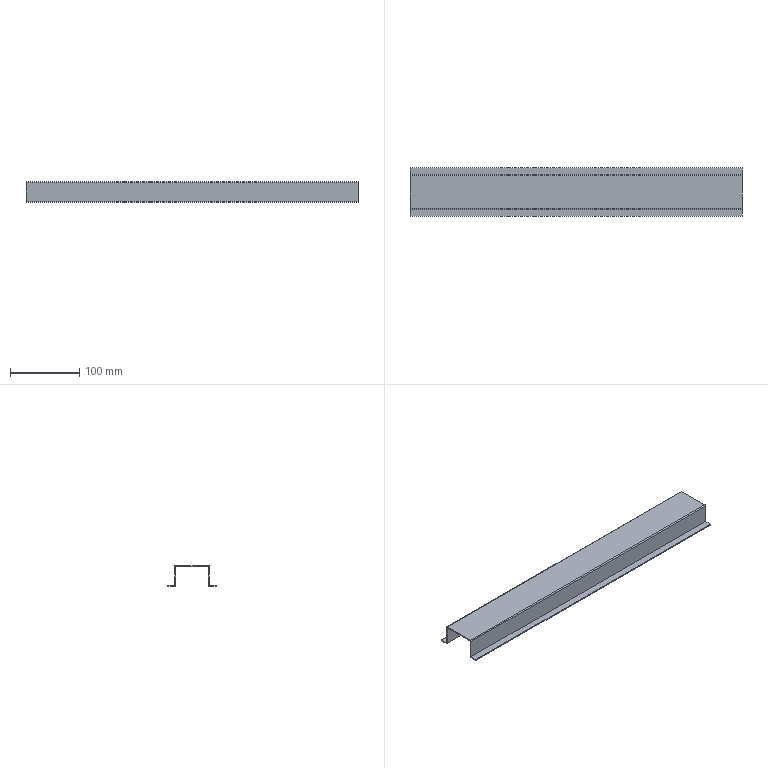Part | STEP file | 1 solid | 18 faces | box 479 x 70 x 30 mm | volume 90339 mm3 | plane 14 | cylinder 4 | commonest cylinder face diameters 3.004 x4
STEP:
#1=CARTESIAN_POINT('',(0.,0.,0.));
#2=DIRECTION('',(0.,0.,1.));
#3=DIRECTION('',(1.,0.,0.));
#4=AXIS2_PLACEMENT_3D('',#1,#2,#3);
#5=CARTESIAN_POINT('',(-1052.573,4254.073,1741.146));
#6=VERTEX_POINT('',#5);
#7=CARTESIAN_POINT('',(-1052.573,4254.073,1768.143));
#8=VERTEX_POINT('',#7);
#9=CARTESIAN_POINT('',(-1052.573,4254.073,1741.146));
#10=DIRECTION('',(0.,0.00002469,1.));
#11=VECTOR('',#10,1.);
#12=LINE('',#9,#11);
#13=CARTESIAN_POINT('',(-1052.573,4302.573,1768.144));
#14=DIRECTION('',(-1.,0.,0.));
#15=DIRECTION('',(0.,0.,1.));
#16=AXIS2_PLACEMENT_3D('',#13,#14,#15);
#17=PLANE('',#16);
#18=CARTESIAN_POINT('',(-26.998,-48.5));
#19=DIRECTION('',(1.,0.00002469));
#20=VECTOR('',#19,1.);
#21=LINE('',#18,#20);
#22=(GEOMETRIC_REPRESENTATION_CONTEXT(2)PARAMETRIC_REPRESENTATION_CONTEXT()REPRESENTATION_CONTEXT('',''));
#23=DEFINITIONAL_REPRESENTATION('',(#21),#22);
#24=PCURVE('',#17,#23);
#25=CARTESIAN_POINT('',(0.,4254.073,0.));
#26=DIRECTION('',(0.,-1.,0.));
#27=DIRECTION('',(0.,0.,-1.));
#28=AXIS2_PLACEMENT_3D('',#25,#26,#27);
#29=PLANE('',#28);
#30=CARTESIAN_POINT('',(-1741.146,-1052.573));
#31=DIRECTION('',(-1.,0.));
#32=VECTOR('',#31,1.);
#33=LINE('',#30,#32);
#34=(GEOMETRIC_REPRESENTATION_CONTEXT(2)PARAMETRIC_REPRESENTATION_CONTEXT()REPRESENTATION_CONTEXT('',''));
#35=DEFINITIONAL_REPRESENTATION('',(#33),#34);
#36=PCURVE('',#29,#35);
#37=SURFACE_CURVE('',#12,(#24,#36),.PCURVE_S1.);
#38=EDGE_CURVE('',#6,#8,#37,.T.);
#39=ORIENTED_EDGE('',*,*,#38,.T.);
#40=CARTESIAN_POINT('',(-1052.573,4301.072,1768.143));
#41=VERTEX_POINT('',#40);
#42=CARTESIAN_POINT('',(-1052.573,4254.073,1768.143));
#43=DIRECTION('',(0.,1.,0.));
#44=VECTOR('',#43,1.);
#45=LINE('',#42,#44);
#46=CARTESIAN_POINT('',(-0.0006667,-48.499));
#47=DIRECTION('',(0.,1.));
#48=VECTOR('',#47,1.);
#49=LINE('',#46,#48);
#50=(GEOMETRIC_REPRESENTATION_CONTEXT(2)PARAMETRIC_REPRESENTATION_CONTEXT()REPRESENTATION_CONTEXT('',''));
#51=DEFINITIONAL_REPRESENTATION('',(#49),#50);
#52=PCURVE('',#17,#51);
#53=CARTESIAN_POINT('',(0.,0.,1768.144));
#54=DIRECTION('',(0.,0.,1.));
#55=DIRECTION('',(1.,0.,0.));
#56=AXIS2_PLACEMENT_3D('',#53,#54,#55);
#57=PLANE('',#56);
#58=CARTESIAN_POINT('',(-1052.573,4254.073));
#59=DIRECTION('',(0.,1.));
#60=VECTOR('',#59,1.);
#61=LINE('',#58,#60);
#62=(GEOMETRIC_REPRESENTATION_CONTEXT(2)PARAMETRIC_REPRESENTATION_CONTEXT()REPRESENTATION_CONTEXT('',''));
#63=DEFINITIONAL_REPRESENTATION('',(#61),#62);
#64=PCURVE('',#57,#63);
#65=SURFACE_CURVE('',#45,(#52,#64),.PCURVE_S1.);
#66=EDGE_CURVE('',#8,#41,#65,.T.);
#67=ORIENTED_EDGE('',*,*,#66,.T.);
#68=CARTESIAN_POINT('',(-1052.573,4301.073,1741.146));
#69=VERTEX_POINT('',#68);
#70=CARTESIAN_POINT('',(-1052.573,4301.073,1741.146));
#71=DIRECTION('',(0.,-0.00002469,1.));
#72=VECTOR('',#71,1.);
#73=LINE('',#70,#72);
#74=CARTESIAN_POINT('',(-26.998,-1.5));
#75=DIRECTION('',(1.,-0.00002469));
#76=VECTOR('',#75,1.);
#77=LINE('',#74,#76);
#78=(GEOMETRIC_REPRESENTATION_CONTEXT(2)PARAMETRIC_REPRESENTATION_CONTEXT()REPRESENTATION_CONTEXT('',''));
#79=DEFINITIONAL_REPRESENTATION('',(#77),#78);
#80=PCURVE('',#17,#79);
#81=CARTESIAN_POINT('',(0.,4301.073,0.));
#82=DIRECTION('',(0.,-1.,0.));
#83=DIRECTION('',(0.,0.,-1.));
#84=AXIS2_PLACEMENT_3D('',#81,#82,#83);
#85=PLANE('',#84);
#86=CARTESIAN_POINT('',(-1741.146,-1052.573));
#87=DIRECTION('',(-1.,0.));
#88=VECTOR('',#87,1.);
#89=LINE('',#86,#88);
#90=(GEOMETRIC_REPRESENTATION_CONTEXT(2)PARAMETRIC_REPRESENTATION_CONTEXT()REPRESENTATION_CONTEXT('',''));
#91=DEFINITIONAL_REPRESENTATION('',(#89),#90);
#92=PCURVE('',#85,#91);
#93=SURFACE_CURVE('',#73,(#80,#92),.PCURVE_S1.);
#94=EDGE_CURVE('',#69,#41,#93,.T.);
#95=ORIENTED_EDGE('',*,*,#94,.F.);
#96=CARTESIAN_POINT('',(-1052.573,4302.575,1739.644));
#97=VERTEX_POINT('',#96);
#98=CARTESIAN_POINT('',(-1052.573,4302.575,1741.146));
#99=DIRECTION('',(-1.,0.,0.));
#100=DIRECTION('',(0.,0.,-1.));
#101=AXIS2_PLACEMENT_3D('',#98,#99,#100);
#102=CIRCLE('',#101,1.502);
#103=CARTESIAN_POINT('',(-26.998,0.002));
#104=DIRECTION('',(-1.,0.));
#105=AXIS2_PLACEMENT_2D('',#103,#104);
#106=CIRCLE('',#105,1.502);
#107=(GEOMETRIC_REPRESENTATION_CONTEXT(2)PARAMETRIC_REPRESENTATION_CONTEXT()REPRESENTATION_CONTEXT('',''));
#108=DEFINITIONAL_REPRESENTATION('',(#106),#107);
#109=PCURVE('',#17,#108);
#110=CARTESIAN_POINT('',(-1052.573,4302.575,1741.146));
#111=DIRECTION('',(1.,0.,0.));
#112=DIRECTION('',(0.,1.,0.));
#113=AXIS2_PLACEMENT_3D('',#110,#111,#112);
#114=CYLINDRICAL_SURFACE('',#113,1.502);
#115=CARTESIAN_POINT('',(4.712,0.));
#116=DIRECTION('',(-1.,0.));
#117=VECTOR('',#116,1.);
#118=LINE('',#115,#117);
#119=(GEOMETRIC_REPRESENTATION_CONTEXT(2)PARAMETRIC_REPRESENTATION_CONTEXT()REPRESENTATION_CONTEXT('',''));
#120=DEFINITIONAL_REPRESENTATION('',(#118),#119);
#121=PCURVE('',#114,#120);
#122=SURFACE_CURVE('',#102,(#109,#121),.PCURVE_S1.);
#123=EDGE_CURVE('',#97,#69,#122,.T.);
#124=ORIENTED_EDGE('',*,*,#123,.F.);
#125=CARTESIAN_POINT('',(-1052.573,4312.573,1739.644));
#126=VERTEX_POINT('',#125);
#127=CARTESIAN_POINT('',(-1052.573,4312.573,1739.644));
#128=DIRECTION('',(0.,-1.,0.));
#129=VECTOR('',#128,1.);
#130=LINE('',#127,#129);
#131=CARTESIAN_POINT('',(-28.5,10.));
#132=DIRECTION('',(0.,-1.));
#133=VECTOR('',#132,1.);
#134=LINE('',#131,#133);
#135=(GEOMETRIC_REPRESENTATION_CONTEXT(2)PARAMETRIC_REPRESENTATION_CONTEXT()REPRESENTATION_CONTEXT('',''));
#136=DEFINITIONAL_REPRESENTATION('',(#134),#135);
#137=PCURVE('',#17,#136);
#138=CARTESIAN_POINT('',(0.,0.,1739.644));
#139=DIRECTION('',(0.,0.,-1.));
#140=DIRECTION('',(-1.,0.,0.));
#141=AXIS2_PLACEMENT_3D('',#138,#139,#140);
#142=PLANE('',#141);
#143=CARTESIAN_POINT('',(1052.573,4312.573));
#144=DIRECTION('',(0.,-1.));
#145=VECTOR('',#144,1.);
#146=LINE('',#143,#145);
#147=(GEOMETRIC_REPRESENTATION_CONTEXT(2)PARAMETRIC_REPRESENTATION_CONTEXT()REPRESENTATION_CONTEXT('',''));
#148=DEFINITIONAL_REPRESENTATION('',(#146),#147);
#149=PCURVE('',#142,#148);
#150=SURFACE_CURVE('',#130,(#137,#149),.PCURVE_S1.);
#151=EDGE_CURVE('',#126,#97,#150,.T.);
#152=ORIENTED_EDGE('',*,*,#151,.F.);
#153=CARTESIAN_POINT('',(-1052.573,4312.573,1741.144));
#154=VERTEX_POINT('',#153);
#155=CARTESIAN_POINT('',(-1052.573,4312.573,1741.144));
#156=DIRECTION('',(0.,0.,-1.));
#157=VECTOR('',#156,1.);
#158=LINE('',#155,#157);
#159=CARTESIAN_POINT('',(-27.,10.));
#160=DIRECTION('',(-1.,0.));
#161=VECTOR('',#160,1.);
#162=LINE('',#159,#161);
#163=(GEOMETRIC_REPRESENTATION_CONTEXT(2)PARAMETRIC_REPRESENTATION_CONTEXT()REPRESENTATION_CONTEXT('',''));
#164=DEFINITIONAL_REPRESENTATION('',(#162),#163);
#165=PCURVE('',#17,#164);
#166=CARTESIAN_POINT('',(-1052.573,4312.573,1739.644));
#167=DIRECTION('',(0.,-1.,0.));
#168=DIRECTION('',(0.,0.,-1.));
#169=AXIS2_PLACEMENT_3D('',#166,#167,#168);
#170=PLANE('',#169);
#171=CARTESIAN_POINT('',(-1.5,0.));
#172=DIRECTION('',(1.,0.));
#173=VECTOR('',#172,1.);
#174=LINE('',#171,#173);
#175=(GEOMETRIC_REPRESENTATION_CONTEXT(2)PARAMETRIC_REPRESENTATION_CONTEXT()REPRESENTATION_CONTEXT('',''));
#176=DEFINITIONAL_REPRESENTATION('',(#174),#175);
#177=PCURVE('',#170,#176);
#178=SURFACE_CURVE('',#158,(#165,#177),.PCURVE_S1.);
#179=EDGE_CURVE('',#154,#126,#178,.T.);
#180=ORIENTED_EDGE('',*,*,#179,.F.);
#181=CARTESIAN_POINT('',(-1052.573,4302.573,1741.144));
#182=VERTEX_POINT('',#181);
#183=CARTESIAN_POINT('',(-1052.573,4312.573,1741.144));
#184=DIRECTION('',(0.,-1.,0.00006667));
#185=VECTOR('',#184,1.);
#186=LINE('',#183,#185);
#187=CARTESIAN_POINT('',(-27.,10.));
#188=DIRECTION('',(0.00006667,-1.));
#189=VECTOR('',#188,1.);
#190=LINE('',#187,#189);
#191=(GEOMETRIC_REPRESENTATION_CONTEXT(2)PARAMETRIC_REPRESENTATION_CONTEXT()REPRESENTATION_CONTEXT('',''));
#192=DEFINITIONAL_REPRESENTATION('',(#190),#191);
#193=PCURVE('',#17,#192);
#194=CARTESIAN_POINT('',(0.,0.,1741.144));
#195=DIRECTION('',(0.,0.,-1.));
#196=DIRECTION('',(-1.,0.,0.));
#197=AXIS2_PLACEMENT_3D('',#194,#195,#196);
#198=PLANE('',#197);
#199=CARTESIAN_POINT('',(1052.573,4312.573));
#200=DIRECTION('',(0.,-1.));
#201=VECTOR('',#200,1.);
#202=LINE('',#199,#201);
#203=(GEOMETRIC_REPRESENTATION_CONTEXT(2)PARAMETRIC_REPRESENTATION_CONTEXT()REPRESENTATION_CONTEXT('',''));
#204=DEFINITIONAL_REPRESENTATION('',(#202),#203);
#205=PCURVE('',#198,#204);
#206=SURFACE_CURVE('',#186,(#193,#205),.PCURVE_S1.);
#207=EDGE_CURVE('',#154,#182,#206,.T.);
#208=ORIENTED_EDGE('',*,*,#207,.T.);
#209=CARTESIAN_POINT('',(-1052.573,4302.573,1768.142));
#210=VERTEX_POINT('',#209);
#211=CARTESIAN_POINT('',(-1052.573,4302.573,1741.144));
#212=DIRECTION('',(0.,-0.00002469,1.));
#213=VECTOR('',#212,1.);
#214=LINE('',#211,#213);
#215=CARTESIAN_POINT('',(-26.999,0.0006667));
#216=DIRECTION('',(1.,-0.00002469));
#217=VECTOR('',#216,1.);
#218=LINE('',#215,#217);
#219=(GEOMETRIC_REPRESENTATION_CONTEXT(2)PARAMETRIC_REPRESENTATION_CONTEXT()REPRESENTATION_CONTEXT('',''));
#220=DEFINITIONAL_REPRESENTATION('',(#218),#219);
#221=PCURVE('',#17,#220);
#222=CARTESIAN_POINT('',(0.,4302.573,0.));
#223=DIRECTION('',(0.,-1.,0.));
#224=DIRECTION('',(0.,0.,-1.));
#225=AXIS2_PLACEMENT_3D('',#222,#223,#224);
#226=PLANE('',#225);
#227=CARTESIAN_POINT('',(-1741.144,-1052.573));
#228=DIRECTION('',(-1.,0.));
#229=VECTOR('',#228,1.);
#230=LINE('',#227,#229);
#231=(GEOMETRIC_REPRESENTATION_CONTEXT(2)PARAMETRIC_REPRESENTATION_CONTEXT()REPRESENTATION_CONTEXT('',''));
#232=DEFINITIONAL_REPRESENTATION('',(#230),#231);
#233=PCURVE('',#226,#232);
#234=SURFACE_CURVE('',#214,(#221,#233),.PCURVE_S1.);
#235=EDGE_CURVE('',#182,#210,#234,.T.);
#236=ORIENTED_EDGE('',*,*,#235,.T.);
#237=CARTESIAN_POINT('',(-1052.573,4301.071,1769.644));
#238=VERTEX_POINT('',#237);
#239=CARTESIAN_POINT('',(-1052.573,4301.071,1768.142));
#240=DIRECTION('',(-1.,0.,0.));
#241=DIRECTION('',(0.,0.,1.));
#242=AXIS2_PLACEMENT_3D('',#239,#240,#241);
#243=CIRCLE('',#242,1.502);
#244=CARTESIAN_POINT('',(-0.002,-1.502));
#245=DIRECTION('',(1.,0.));
#246=AXIS2_PLACEMENT_2D('',#244,#245);
#247=CIRCLE('',#246,1.502);
#248=(GEOMETRIC_REPRESENTATION_CONTEXT(2)PARAMETRIC_REPRESENTATION_CONTEXT()REPRESENTATION_CONTEXT('',''));
#249=DEFINITIONAL_REPRESENTATION('',(#247),#248);
#250=PCURVE('',#17,#249);
#251=CARTESIAN_POINT('',(-573.573,4301.071,1768.142));
#252=DIRECTION('',(-1.,0.,0.));
#253=DIRECTION('',(0.,0.,-1.));
#254=AXIS2_PLACEMENT_3D('',#251,#252,#253);
#255=CYLINDRICAL_SURFACE('',#254,1.502);
#256=CARTESIAN_POINT('',(3.142,479.));
#257=DIRECTION('',(1.,0.));
#258=VECTOR('',#257,1.);
#259=LINE('',#256,#258);
#260=(GEOMETRIC_REPRESENTATION_CONTEXT(2)PARAMETRIC_REPRESENTATION_CONTEXT()REPRESENTATION_CONTEXT('',''));
#261=DEFINITIONAL_REPRESENTATION('',(#259),#260);
#262=PCURVE('',#255,#261);
#263=SURFACE_CURVE('',#243,(#250,#262),.PCURVE_S1.);
#264=EDGE_CURVE('',#238,#210,#263,.T.);
#265=ORIENTED_EDGE('',*,*,#264,.F.);
#266=CARTESIAN_POINT('',(-1052.573,4254.075,1769.644));
#267=VERTEX_POINT('',#266);
#268=CARTESIAN_POINT('',(-1052.573,4254.075,1769.644));
#269=DIRECTION('',(0.,1.,0.));
#270=VECTOR('',#269,1.);
#271=LINE('',#268,#270);
#272=CARTESIAN_POINT('',(1.5,-48.498));
#273=DIRECTION('',(0.,1.));
#274=VECTOR('',#273,1.);
#275=LINE('',#272,#274);
#276=(GEOMETRIC_REPRESENTATION_CONTEXT(2)PARAMETRIC_REPRESENTATION_CONTEXT()REPRESENTATION_CONTEXT('',''));
#277=DEFINITIONAL_REPRESENTATION('',(#275),#276);
#278=PCURVE('',#17,#277);
#279=CARTESIAN_POINT('',(0.,0.,1769.644));
#280=DIRECTION('',(0.,0.,1.));
#281=DIRECTION('',(1.,0.,0.));
#282=AXIS2_PLACEMENT_3D('',#279,#280,#281);
#283=PLANE('',#282);
#284=CARTESIAN_POINT('',(-1052.573,4254.075));
#285=DIRECTION('',(0.,1.));
#286=VECTOR('',#285,1.);
#287=LINE('',#284,#286);
#288=(GEOMETRIC_REPRESENTATION_CONTEXT(2)PARAMETRIC_REPRESENTATION_CONTEXT()REPRESENTATION_CONTEXT('',''));
#289=DEFINITIONAL_REPRESENTATION('',(#287),#288);
#290=PCURVE('',#283,#289);
#291=SURFACE_CURVE('',#271,(#278,#290),.PCURVE_S1.);
#292=EDGE_CURVE('',#267,#238,#291,.T.);
#293=ORIENTED_EDGE('',*,*,#292,.F.);
#294=CARTESIAN_POINT('',(-1052.573,4252.573,1768.142));
#295=VERTEX_POINT('',#294);
#296=CARTESIAN_POINT('',(-1052.573,4254.075,1768.142));
#297=DIRECTION('',(-1.,0.,0.));
#298=DIRECTION('',(0.,-1.,0.));
#299=AXIS2_PLACEMENT_3D('',#296,#297,#298);
#300=CIRCLE('',#299,1.502);
#301=CARTESIAN_POINT('',(-0.002,-48.498));
#302=DIRECTION('',(0.,-1.));
#303=AXIS2_PLACEMENT_2D('',#301,#302);
#304=CIRCLE('',#303,1.502);
#305=(GEOMETRIC_REPRESENTATION_CONTEXT(2)PARAMETRIC_REPRESENTATION_CONTEXT()REPRESENTATION_CONTEXT('',''));
#306=DEFINITIONAL_REPRESENTATION('',(#304),#305);
#307=PCURVE('',#17,#306);
#308=CARTESIAN_POINT('',(-1052.573,4254.075,1768.142));
#309=DIRECTION('',(1.,0.,0.));
#310=DIRECTION('',(0.,0.,-1.));
#311=AXIS2_PLACEMENT_3D('',#308,#309,#310);
#312=CYLINDRICAL_SURFACE('',#311,1.502);
#313=CARTESIAN_POINT('',(4.712,0.));
#314=DIRECTION('',(-1.,0.));
#315=VECTOR('',#314,1.);
#316=LINE('',#313,#315);
#317=(GEOMETRIC_REPRESENTATION_CONTEXT(2)PARAMETRIC_REPRESENTATION_CONTEXT()REPRESENTATION_CONTEXT('',''));
#318=DEFINITIONAL_REPRESENTATION('',(#316),#317);
#319=PCURVE('',#312,#318);
#320=SURFACE_CURVE('',#300,(#307,#319),.PCURVE_S1.);
#321=EDGE_CURVE('',#295,#267,#320,.T.);
#322=ORIENTED_EDGE('',*,*,#321,.F.);
#323=CARTESIAN_POINT('',(-1052.573,4252.572,1741.144));
#324=VERTEX_POINT('',#323);
#325=CARTESIAN_POINT('',(-1052.573,4252.572,1741.144));
#326=DIRECTION('',(0.,0.00002469,1.));
#327=VECTOR('',#326,1.);
#328=LINE('',#325,#327);
#329=CARTESIAN_POINT('',(-26.999,-50.001));
#330=DIRECTION('',(1.,0.00002469));
#331=VECTOR('',#330,1.);
#332=LINE('',#329,#331);
#333=(GEOMETRIC_REPRESENTATION_CONTEXT(2)PARAMETRIC_REPRESENTATION_CONTEXT()REPRESENTATION_CONTEXT('',''));
#334=DEFINITIONAL_REPRESENTATION('',(#332),#333);
#335=PCURVE('',#17,#334);
#336=CARTESIAN_POINT('',(0.,4252.573,0.));
#337=DIRECTION('',(0.,-1.,0.));
#338=DIRECTION('',(0.,0.,-1.));
#339=AXIS2_PLACEMENT_3D('',#336,#337,#338);
#340=PLANE('',#339);
#341=CARTESIAN_POINT('',(-1741.144,-1052.573));
#342=DIRECTION('',(-1.,0.));
#343=VECTOR('',#342,1.);
#344=LINE('',#341,#343);
#345=(GEOMETRIC_REPRESENTATION_CONTEXT(2)PARAMETRIC_REPRESENTATION_CONTEXT()REPRESENTATION_CONTEXT('',''));
#346=DEFINITIONAL_REPRESENTATION('',(#344),#345);
#347=PCURVE('',#340,#346);
#348=SURFACE_CURVE('',#328,(#335,#347),.PCURVE_S1.);
#349=EDGE_CURVE('',#324,#295,#348,.T.);
#350=ORIENTED_EDGE('',*,*,#349,.F.);
#351=CARTESIAN_POINT('',(-1052.573,4242.573,1741.144));
#352=VERTEX_POINT('',#351);
#353=CARTESIAN_POINT('',(-1052.573,4242.573,1741.144));
#354=DIRECTION('',(0.,1.,0.00006667));
#355=VECTOR('',#354,1.);
#356=LINE('',#353,#355);
#357=CARTESIAN_POINT('',(-27.,-60.));
#358=DIRECTION('',(0.00006667,1.));
#359=VECTOR('',#358,1.);
#360=LINE('',#357,#359);
#361=(GEOMETRIC_REPRESENTATION_CONTEXT(2)PARAMETRIC_REPRESENTATION_CONTEXT()REPRESENTATION_CONTEXT('',''));
#362=DEFINITIONAL_REPRESENTATION('',(#360),#361);
#363=PCURVE('',#17,#362);
#364=CARTESIAN_POINT('',(0.,0.,1741.144));
#365=DIRECTION('',(0.,0.,1.));
#366=DIRECTION('',(1.,0.,0.));
#367=AXIS2_PLACEMENT_3D('',#364,#365,#366);
#368=PLANE('',#367);
#369=CARTESIAN_POINT('',(-1052.573,4242.573));
#370=DIRECTION('',(0.,1.));
#371=VECTOR('',#370,1.);
#372=LINE('',#369,#371);
#373=(GEOMETRIC_REPRESENTATION_CONTEXT(2)PARAMETRIC_REPRESENTATION_CONTEXT()REPRESENTATION_CONTEXT('',''));
#374=DEFINITIONAL_REPRESENTATION('',(#372),#373);
#375=PCURVE('',#368,#374);
#376=SURFACE_CURVE('',#356,(#363,#375),.PCURVE_S1.);
#377=EDGE_CURVE('',#352,#324,#376,.T.);
#378=ORIENTED_EDGE('',*,*,#377,.F.);
#379=CARTESIAN_POINT('',(-1052.573,4242.573,1739.644));
#380=VERTEX_POINT('',#379);
#381=CARTESIAN_POINT('',(-1052.573,4242.573,1741.144));
#382=DIRECTION('',(0.,0.,-1.));
#383=VECTOR('',#382,1.);
#384=LINE('',#381,#383);
#385=CARTESIAN_POINT('',(-27.,-60.));
#386=DIRECTION('',(-1.,0.));
#387=VECTOR('',#386,1.);
#388=LINE('',#385,#387);
#389=(GEOMETRIC_REPRESENTATION_CONTEXT(2)PARAMETRIC_REPRESENTATION_CONTEXT()REPRESENTATION_CONTEXT('',''));
#390=DEFINITIONAL_REPRESENTATION('',(#388),#389);
#391=PCURVE('',#17,#390);
#392=CARTESIAN_POINT('',(-1052.573,4242.573,1739.644));
#393=DIRECTION('',(0.,-1.,0.));
#394=DIRECTION('',(0.,0.,-1.));
#395=AXIS2_PLACEMENT_3D('',#392,#393,#394);
#396=PLANE('',#395);
#397=CARTESIAN_POINT('',(-1.5,0.));
#398=DIRECTION('',(1.,0.));
#399=VECTOR('',#398,1.);
#400=LINE('',#397,#399);
#401=(GEOMETRIC_REPRESENTATION_CONTEXT(2)PARAMETRIC_REPRESENTATION_CONTEXT()REPRESENTATION_CONTEXT('',''));
#402=DEFINITIONAL_REPRESENTATION('',(#400),#401);
#403=PCURVE('',#396,#402);
#404=SURFACE_CURVE('',#384,(#391,#403),.PCURVE_S1.);
#405=EDGE_CURVE('',#352,#380,#404,.T.);
#406=ORIENTED_EDGE('',*,*,#405,.T.);
#407=CARTESIAN_POINT('',(-1052.573,4252.571,1739.644));
#408=VERTEX_POINT('',#407);
#409=CARTESIAN_POINT('',(-1052.573,4242.573,1739.644));
#410=DIRECTION('',(0.,1.,0.));
#411=VECTOR('',#410,1.);
#412=LINE('',#409,#411);
#413=CARTESIAN_POINT('',(-28.5,-60.));
#414=DIRECTION('',(0.,1.));
#415=VECTOR('',#414,1.);
#416=LINE('',#413,#415);
#417=(GEOMETRIC_REPRESENTATION_CONTEXT(2)PARAMETRIC_REPRESENTATION_CONTEXT()REPRESENTATION_CONTEXT('',''));
#418=DEFINITIONAL_REPRESENTATION('',(#416),#417);
#419=PCURVE('',#17,#418);
#420=CARTESIAN_POINT('',(0.,0.,1739.644));
#421=DIRECTION('',(0.,0.,1.));
#422=DIRECTION('',(1.,0.,0.));
#423=AXIS2_PLACEMENT_3D('',#420,#421,#422);
#424=PLANE('',#423);
#425=CARTESIAN_POINT('',(-1052.573,4242.573));
#426=DIRECTION('',(0.,1.));
#427=VECTOR('',#426,1.);
#428=LINE('',#425,#427);
#429=(GEOMETRIC_REPRESENTATION_CONTEXT(2)PARAMETRIC_REPRESENTATION_CONTEXT()REPRESENTATION_CONTEXT('',''));
#430=DEFINITIONAL_REPRESENTATION('',(#428),#429);
#431=PCURVE('',#424,#430);
#432=SURFACE_CURVE('',#412,(#419,#431),.PCURVE_S1.);
#433=EDGE_CURVE('',#380,#408,#432,.T.);
#434=ORIENTED_EDGE('',*,*,#433,.T.);
#435=CARTESIAN_POINT('',(-1052.573,4252.571,1741.146));
#436=DIRECTION('',(-1.,0.,0.));
#437=DIRECTION('',(0.,1.,0.));
#438=AXIS2_PLACEMENT_3D('',#435,#436,#437);
#439=CIRCLE('',#438,1.502);
#440=CARTESIAN_POINT('',(-26.998,-50.002));
#441=DIRECTION('',(0.,1.));
#442=AXIS2_PLACEMENT_2D('',#440,#441);
#443=CIRCLE('',#442,1.502);
#444=(GEOMETRIC_REPRESENTATION_CONTEXT(2)PARAMETRIC_REPRESENTATION_CONTEXT()REPRESENTATION_CONTEXT('',''));
#445=DEFINITIONAL_REPRESENTATION('',(#443),#444);
#446=PCURVE('',#17,#445);
#447=CARTESIAN_POINT('',(-573.573,4252.571,1741.146));
#448=DIRECTION('',(-1.,0.,0.));
#449=DIRECTION('',(0.,-1.,0.));
#450=AXIS2_PLACEMENT_3D('',#447,#448,#449);
#451=CYLINDRICAL_SURFACE('',#450,1.502);
#452=CARTESIAN_POINT('',(3.142,479.));
#453=DIRECTION('',(1.,0.));
#454=VECTOR('',#453,1.);
#455=LINE('',#452,#454);
#456=(GEOMETRIC_REPRESENTATION_CONTEXT(2)PARAMETRIC_REPRESENTATION_CONTEXT()REPRESENTATION_CONTEXT('',''));
#457=DEFINITIONAL_REPRESENTATION('',(#455),#456);
#458=PCURVE('',#451,#457);
#459=SURFACE_CURVE('',#439,(#446,#458),.PCURVE_S1.);
#460=EDGE_CURVE('',#6,#408,#459,.T.);
#461=ORIENTED_EDGE('',*,*,#460,.F.);
#462=EDGE_LOOP('',(#39,#67,#95,#124,#152,#180,#208,#236,#265,#293,#322,#350,#378,#406,#434,#461));
#463=FACE_BOUND('',#462,.F.);
#464=ADVANCED_FACE('',(#463),#17,.T.);
#465=CARTESIAN_POINT('',(-573.573,4254.073,1768.143));
#466=VERTEX_POINT('',#465);
#467=CARTESIAN_POINT('',(-573.573,4254.073,1741.146));
#468=VERTEX_POINT('',#467);
#469=CARTESIAN_POINT('',(-573.573,4254.073,1768.143));
#470=DIRECTION('',(0.,-0.00002469,-1.));
#471=VECTOR('',#470,1.);
#472=LINE('',#469,#471);
#473=CARTESIAN_POINT('',(-1768.143,-573.573));
#474=DIRECTION('',(1.,0.));
#475=VECTOR('',#474,1.);
#476=LINE('',#473,#475);
#477=(GEOMETRIC_REPRESENTATION_CONTEXT(2)PARAMETRIC_REPRESENTATION_CONTEXT()REPRESENTATION_CONTEXT('',''));
#478=DEFINITIONAL_REPRESENTATION('',(#476),#477);
#479=PCURVE('',#29,#478);
#480=CARTESIAN_POINT('',(-573.573,4252.573,1768.144));
#481=DIRECTION('',(1.,0.,0.));
#482=DIRECTION('',(0.,0.,-1.));
#483=AXIS2_PLACEMENT_3D('',#480,#481,#482);
#484=PLANE('',#483);
#485=CARTESIAN_POINT('',(0.0006667,1.501));
#486=DIRECTION('',(1.,-0.00002469));
#487=VECTOR('',#486,1.);
#488=LINE('',#485,#487);
#489=(GEOMETRIC_REPRESENTATION_CONTEXT(2)PARAMETRIC_REPRESENTATION_CONTEXT()REPRESENTATION_CONTEXT('',''));
#490=DEFINITIONAL_REPRESENTATION('',(#488),#489);
#491=PCURVE('',#484,#490);
#492=SURFACE_CURVE('',#472,(#479,#491),.PCURVE_S1.);
#493=EDGE_CURVE('',#466,#468,#492,.T.);
#494=ORIENTED_EDGE('',*,*,#493,.F.);
#495=CARTESIAN_POINT('',(-573.573,4254.073,1768.143));
#496=DIRECTION('',(-1.,0.,0.));
#497=VECTOR('',#496,1.);
#498=LINE('',#495,#497);
#499=CARTESIAN_POINT('',(-1768.143,-573.573));
#500=DIRECTION('',(0.,-1.));
#501=VECTOR('',#500,1.);
#502=LINE('',#499,#501);
#503=(GEOMETRIC_REPRESENTATION_CONTEXT(2)PARAMETRIC_REPRESENTATION_CONTEXT()REPRESENTATION_CONTEXT('',''));
#504=DEFINITIONAL_REPRESENTATION('',(#502),#503);
#505=PCURVE('',#29,#504);
#506=CARTESIAN_POINT('',(-573.573,4254.073));
#507=DIRECTION('',(-1.,0.));
#508=VECTOR('',#507,1.);
#509=LINE('',#506,#508);
#510=(GEOMETRIC_REPRESENTATION_CONTEXT(2)PARAMETRIC_REPRESENTATION_CONTEXT()REPRESENTATION_CONTEXT('',''));
#511=DEFINITIONAL_REPRESENTATION('',(#509),#510);
#512=PCURVE('',#57,#511);
#513=SURFACE_CURVE('',#498,(#505,#512),.PCURVE_S1.);
#514=EDGE_CURVE('',#466,#8,#513,.T.);
#515=ORIENTED_EDGE('',*,*,#514,.T.);
#516=ORIENTED_EDGE('',*,*,#38,.F.);
#517=CARTESIAN_POINT('',(-1052.573,4254.073,1741.146));
#518=DIRECTION('',(1.,0.,0.));
#519=VECTOR('',#518,1.);
#520=LINE('',#517,#519);
#521=CARTESIAN_POINT('',(-1741.146,-1052.573));
#522=DIRECTION('',(0.,1.));
#523=VECTOR('',#522,1.);
#524=LINE('',#521,#523);
#525=(GEOMETRIC_REPRESENTATION_CONTEXT(2)PARAMETRIC_REPRESENTATION_CONTEXT()REPRESENTATION_CONTEXT('',''));
#526=DEFINITIONAL_REPRESENTATION('',(#524),#525);
#527=PCURVE('',#29,#526);
#528=CARTESIAN_POINT('',(3.142,479.));
#529=DIRECTION('',(0.,-1.));
#530=VECTOR('',#529,1.);
#531=LINE('',#528,#530);
#532=(GEOMETRIC_REPRESENTATION_CONTEXT(2)PARAMETRIC_REPRESENTATION_CONTEXT()REPRESENTATION_CONTEXT('',''));
#533=DEFINITIONAL_REPRESENTATION('',(#531),#532);
#534=PCURVE('',#451,#533);
#535=SURFACE_CURVE('',#520,(#527,#534),.PCURVE_S1.);
#536=EDGE_CURVE('',#6,#468,#535,.T.);
#537=ORIENTED_EDGE('',*,*,#536,.T.);
#538=EDGE_LOOP('',(#494,#515,#516,#537));
#539=FACE_BOUND('',#538,.F.);
#540=ADVANCED_FACE('',(#539),#29,.F.);
#541=CARTESIAN_POINT('',(-573.573,4252.573,1768.142));
#542=VERTEX_POINT('',#541);
#543=CARTESIAN_POINT('',(-573.573,4252.572,1741.144));
#544=VERTEX_POINT('',#543);
#545=CARTESIAN_POINT('',(-573.573,4252.573,1768.142));
#546=DIRECTION('',(0.,-0.00002469,-1.));
#547=VECTOR('',#546,1.);
#548=LINE('',#545,#547);
#549=CARTESIAN_POINT('',(0.002,0.));
#550=DIRECTION('',(1.,-0.00002469));
#551=VECTOR('',#550,1.);
#552=LINE('',#549,#551);
#553=(GEOMETRIC_REPRESENTATION_CONTEXT(2)PARAMETRIC_REPRESENTATION_CONTEXT()REPRESENTATION_CONTEXT('',''));
#554=DEFINITIONAL_REPRESENTATION('',(#552),#553);
#555=PCURVE('',#484,#554);
#556=CARTESIAN_POINT('',(-1768.142,-573.573));
#557=DIRECTION('',(1.,0.));
#558=VECTOR('',#557,1.);
#559=LINE('',#556,#558);
#560=(GEOMETRIC_REPRESENTATION_CONTEXT(2)PARAMETRIC_REPRESENTATION_CONTEXT()REPRESENTATION_CONTEXT('',''));
#561=DEFINITIONAL_REPRESENTATION('',(#559),#560);
#562=PCURVE('',#340,#561);
#563=SURFACE_CURVE('',#548,(#555,#562),.PCURVE_S1.);
#564=EDGE_CURVE('',#542,#544,#563,.T.);
#565=ORIENTED_EDGE('',*,*,#564,.F.);
#566=CARTESIAN_POINT('',(-573.573,4254.075,1769.644));
#567=VERTEX_POINT('',#566);
#568=CARTESIAN_POINT('',(-573.573,4254.075,1768.142));
#569=DIRECTION('',(1.,0.,0.));
#570=DIRECTION('',(0.,0.,1.));
#571=AXIS2_PLACEMENT_3D('',#568,#569,#570);
#572=CIRCLE('',#571,1.502);
#573=CARTESIAN_POINT('',(0.002,1.502));
#574=DIRECTION('',(-1.,0.));
#575=AXIS2_PLACEMENT_2D('',#573,#574);
#576=CIRCLE('',#575,1.502);
#577=(GEOMETRIC_REPRESENTATION_CONTEXT(2)PARAMETRIC_REPRESENTATION_CONTEXT()REPRESENTATION_CONTEXT('',''));
#578=DEFINITIONAL_REPRESENTATION('',(#576),#577);
#579=PCURVE('',#484,#578);
#580=CARTESIAN_POINT('',(3.142,479.));
#581=DIRECTION('',(1.,0.));
#582=VECTOR('',#581,1.);
#583=LINE('',#580,#582);
#584=(GEOMETRIC_REPRESENTATION_CONTEXT(2)PARAMETRIC_REPRESENTATION_CONTEXT()REPRESENTATION_CONTEXT('',''));
#585=DEFINITIONAL_REPRESENTATION('',(#583),#584);
#586=PCURVE('',#312,#585);
#587=SURFACE_CURVE('',#572,(#579,#586),.PCURVE_S1.);
#588=EDGE_CURVE('',#567,#542,#587,.T.);
#589=ORIENTED_EDGE('',*,*,#588,.F.);
#590=CARTESIAN_POINT('',(-573.573,4301.071,1769.644));
#591=VERTEX_POINT('',#590);
#592=CARTESIAN_POINT('',(-573.573,4301.071,1769.644));
#593=DIRECTION('',(0.,-1.,0.));
#594=VECTOR('',#593,1.);
#595=LINE('',#592,#594);
#596=CARTESIAN_POINT('',(-1.5,48.498));
#597=DIRECTION('',(0.,-1.));
#598=VECTOR('',#597,1.);
#599=LINE('',#596,#598);
#600=(GEOMETRIC_REPRESENTATION_CONTEXT(2)PARAMETRIC_REPRESENTATION_CONTEXT()REPRESENTATION_CONTEXT('',''));
#601=DEFINITIONAL_REPRESENTATION('',(#599),#600);
#602=PCURVE('',#484,#601);
#603=CARTESIAN_POINT('',(-573.573,4301.071));
#604=DIRECTION('',(0.,-1.));
#605=VECTOR('',#604,1.);
#606=LINE('',#603,#605);
#607=(GEOMETRIC_REPRESENTATION_CONTEXT(2)PARAMETRIC_REPRESENTATION_CONTEXT()REPRESENTATION_CONTEXT('',''));
#608=DEFINITIONAL_REPRESENTATION('',(#606),#607);
#609=PCURVE('',#283,#608);
#610=SURFACE_CURVE('',#595,(#602,#609),.PCURVE_S1.);
#611=EDGE_CURVE('',#591,#567,#610,.T.);
#612=ORIENTED_EDGE('',*,*,#611,.F.);
#613=CARTESIAN_POINT('',(-573.573,4302.573,1768.142));
#614=VERTEX_POINT('',#613);
#615=CARTESIAN_POINT('',(-573.573,4301.071,1768.142));
#616=DIRECTION('',(1.,0.,0.));
#617=DIRECTION('',(0.,1.,0.));
#618=AXIS2_PLACEMENT_3D('',#615,#616,#617);
#619=CIRCLE('',#618,1.502);
#620=CARTESIAN_POINT('',(0.002,48.498));
#621=DIRECTION('',(0.,1.));
#622=AXIS2_PLACEMENT_2D('',#620,#621);
#623=CIRCLE('',#622,1.502);
#624=(GEOMETRIC_REPRESENTATION_CONTEXT(2)PARAMETRIC_REPRESENTATION_CONTEXT()REPRESENTATION_CONTEXT('',''));
#625=DEFINITIONAL_REPRESENTATION('',(#623),#624);
#626=PCURVE('',#484,#625);
#627=CARTESIAN_POINT('',(4.712,0.));
#628=DIRECTION('',(-1.,0.));
#629=VECTOR('',#628,1.);
#630=LINE('',#627,#629);
#631=(GEOMETRIC_REPRESENTATION_CONTEXT(2)PARAMETRIC_REPRESENTATION_CONTEXT()REPRESENTATION_CONTEXT('',''));
#632=DEFINITIONAL_REPRESENTATION('',(#630),#631);
#633=PCURVE('',#255,#632);
#634=SURFACE_CURVE('',#619,(#626,#633),.PCURVE_S1.);
#635=EDGE_CURVE('',#614,#591,#634,.T.);
#636=ORIENTED_EDGE('',*,*,#635,.F.);
#637=CARTESIAN_POINT('',(-573.573,4302.573,1741.144));
#638=VERTEX_POINT('',#637);
#639=CARTESIAN_POINT('',(-573.573,4302.573,1768.142));
#640=DIRECTION('',(0.,0.00002469,-1.));
#641=VECTOR('',#640,1.);
#642=LINE('',#639,#641);
#643=CARTESIAN_POINT('',(0.002,50.));
#644=DIRECTION('',(1.,0.00002469));
#645=VECTOR('',#644,1.);
#646=LINE('',#643,#645);
#647=(GEOMETRIC_REPRESENTATION_CONTEXT(2)PARAMETRIC_REPRESENTATION_CONTEXT()REPRESENTATION_CONTEXT('',''));
#648=DEFINITIONAL_REPRESENTATION('',(#646),#647);
#649=PCURVE('',#484,#648);
#650=CARTESIAN_POINT('',(-1768.142,-573.573));
#651=DIRECTION('',(1.,0.));
#652=VECTOR('',#651,1.);
#653=LINE('',#650,#652);
#654=(GEOMETRIC_REPRESENTATION_CONTEXT(2)PARAMETRIC_REPRESENTATION_CONTEXT()REPRESENTATION_CONTEXT('',''));
#655=DEFINITIONAL_REPRESENTATION('',(#653),#654);
#656=PCURVE('',#226,#655);
#657=SURFACE_CURVE('',#642,(#649,#656),.PCURVE_S1.);
#658=EDGE_CURVE('',#614,#638,#657,.T.);
#659=ORIENTED_EDGE('',*,*,#658,.T.);
#660=CARTESIAN_POINT('',(-573.573,4312.573,1741.144));
#661=VERTEX_POINT('',#660);
#662=CARTESIAN_POINT('',(-573.573,4302.573,1741.144));
#663=DIRECTION('',(0.,1.,-0.00006667));
#664=VECTOR('',#663,1.);
#665=LINE('',#662,#664);
#666=CARTESIAN_POINT('',(26.999,50.001));
#667=DIRECTION('',(0.00006667,1.));
#668=VECTOR('',#667,1.);
#669=LINE('',#666,#668);
#670=(GEOMETRIC_REPRESENTATION_CONTEXT(2)PARAMETRIC_REPRESENTATION_CONTEXT()REPRESENTATION_CONTEXT('',''));
#671=DEFINITIONAL_REPRESENTATION('',(#669),#670);
#672=PCURVE('',#484,#671);
#673=CARTESIAN_POINT('',(573.573,4302.573));
#674=DIRECTION('',(0.,1.));
#675=VECTOR('',#674,1.);
#676=LINE('',#673,#675);
#677=(GEOMETRIC_REPRESENTATION_CONTEXT(2)PARAMETRIC_REPRESENTATION_CONTEXT()REPRESENTATION_CONTEXT('',''));
#678=DEFINITIONAL_REPRESENTATION('',(#676),#677);
#679=PCURVE('',#198,#678);
#680=SURFACE_CURVE('',#665,(#672,#679),.PCURVE_S1.);
#681=EDGE_CURVE('',#638,#661,#680,.T.);
#682=ORIENTED_EDGE('',*,*,#681,.T.);
#683=CARTESIAN_POINT('',(-573.573,4312.573,1739.644));
#684=VERTEX_POINT('',#683);
#685=CARTESIAN_POINT('',(-573.573,4312.573,1741.144));
#686=DIRECTION('',(0.,0.,-1.));
#687=VECTOR('',#686,1.);
#688=LINE('',#685,#687);
#689=CARTESIAN_POINT('',(27.,60.));
#690=DIRECTION('',(1.,0.));
#691=VECTOR('',#690,1.);
#692=LINE('',#689,#691);
#693=(GEOMETRIC_REPRESENTATION_CONTEXT(2)PARAMETRIC_REPRESENTATION_CONTEXT()REPRESENTATION_CONTEXT('',''));
#694=DEFINITIONAL_REPRESENTATION('',(#692),#693);
#695=PCURVE('',#484,#694);
#696=CARTESIAN_POINT('',(-1.5,479.));
#697=DIRECTION('',(1.,0.));
#698=VECTOR('',#697,1.);
#699=LINE('',#696,#698);
#700=(GEOMETRIC_REPRESENTATION_CONTEXT(2)PARAMETRIC_REPRESENTATION_CONTEXT()REPRESENTATION_CONTEXT('',''));
#701=DEFINITIONAL_REPRESENTATION('',(#699),#700);
#702=PCURVE('',#170,#701);
#703=SURFACE_CURVE('',#688,(#695,#702),.PCURVE_S1.);
#704=EDGE_CURVE('',#661,#684,#703,.T.);
#705=ORIENTED_EDGE('',*,*,#704,.T.);
#706=CARTESIAN_POINT('',(-573.573,4302.575,1739.644));
#707=VERTEX_POINT('',#706);
#708=CARTESIAN_POINT('',(-573.573,4302.575,1739.644));
#709=DIRECTION('',(0.,1.,0.));
#710=VECTOR('',#709,1.);
#711=LINE('',#708,#710);
#712=CARTESIAN_POINT('',(28.5,50.002));
#713=DIRECTION('',(0.,1.));
#714=VECTOR('',#713,1.);
#715=LINE('',#712,#714);
#716=(GEOMETRIC_REPRESENTATION_CONTEXT(2)PARAMETRIC_REPRESENTATION_CONTEXT()REPRESENTATION_CONTEXT('',''));
#717=DEFINITIONAL_REPRESENTATION('',(#715),#716);
#718=PCURVE('',#484,#717);
#719=CARTESIAN_POINT('',(573.573,4302.575));
#720=DIRECTION('',(0.,1.));
#721=VECTOR('',#720,1.);
#722=LINE('',#719,#721);
#723=(GEOMETRIC_REPRESENTATION_CONTEXT(2)PARAMETRIC_REPRESENTATION_CONTEXT()REPRESENTATION_CONTEXT('',''));
#724=DEFINITIONAL_REPRESENTATION('',(#722),#723);
#725=PCURVE('',#142,#724);
#726=SURFACE_CURVE('',#711,(#718,#725),.PCURVE_S1.);
#727=EDGE_CURVE('',#707,#684,#726,.T.);
#728=ORIENTED_EDGE('',*,*,#727,.F.);
#729=CARTESIAN_POINT('',(-573.573,4301.073,1741.146));
#730=VERTEX_POINT('',#729);
#731=CARTESIAN_POINT('',(-573.573,4302.575,1741.146));
#732=DIRECTION('',(1.,0.,0.));
#733=DIRECTION('',(0.,-1.,0.));
#734=AXIS2_PLACEMENT_3D('',#731,#732,#733);
#735=CIRCLE('',#734,1.502);
#736=CARTESIAN_POINT('',(26.998,50.002));
#737=DIRECTION('',(0.,-1.));
#738=AXIS2_PLACEMENT_2D('',#736,#737);
#739=CIRCLE('',#738,1.502);
#740=(GEOMETRIC_REPRESENTATION_CONTEXT(2)PARAMETRIC_REPRESENTATION_CONTEXT()REPRESENTATION_CONTEXT('',''));
#741=DEFINITIONAL_REPRESENTATION('',(#739),#740);
#742=PCURVE('',#484,#741);
#743=CARTESIAN_POINT('',(3.142,479.));
#744=DIRECTION('',(1.,0.));
#745=VECTOR('',#744,1.);
#746=LINE('',#743,#745);
#747=(GEOMETRIC_REPRESENTATION_CONTEXT(2)PARAMETRIC_REPRESENTATION_CONTEXT()REPRESENTATION_CONTEXT('',''));
#748=DEFINITIONAL_REPRESENTATION('',(#746),#747);
#749=PCURVE('',#114,#748);
#750=SURFACE_CURVE('',#735,(#742,#749),.PCURVE_S1.);
#751=EDGE_CURVE('',#730,#707,#750,.T.);
#752=ORIENTED_EDGE('',*,*,#751,.F.);
#753=CARTESIAN_POINT('',(-573.573,4301.072,1768.143));
#754=VERTEX_POINT('',#753);
#755=CARTESIAN_POINT('',(-573.573,4301.072,1768.143));
#756=DIRECTION('',(0.,0.00002469,-1.));
#757=VECTOR('',#756,1.);
#758=LINE('',#755,#757);
#759=CARTESIAN_POINT('',(0.0006667,48.499));
#760=DIRECTION('',(1.,0.00002469));
#761=VECTOR('',#760,1.);
#762=LINE('',#759,#761);
#763=(GEOMETRIC_REPRESENTATION_CONTEXT(2)PARAMETRIC_REPRESENTATION_CONTEXT()REPRESENTATION_CONTEXT('',''));
#764=DEFINITIONAL_REPRESENTATION('',(#762),#763);
#765=PCURVE('',#484,#764);
#766=CARTESIAN_POINT('',(-1768.143,-573.573));
#767=DIRECTION('',(1.,0.));
#768=VECTOR('',#767,1.);
#769=LINE('',#766,#768);
#770=(GEOMETRIC_REPRESENTATION_CONTEXT(2)PARAMETRIC_REPRESENTATION_CONTEXT()REPRESENTATION_CONTEXT('',''));
#771=DEFINITIONAL_REPRESENTATION('',(#769),#770);
#772=PCURVE('',#85,#771);
#773=SURFACE_CURVE('',#758,(#765,#772),.PCURVE_S1.);
#774=EDGE_CURVE('',#754,#730,#773,.T.);
#775=ORIENTED_EDGE('',*,*,#774,.F.);
#776=CARTESIAN_POINT('',(-573.573,4301.072,1768.143));
#777=DIRECTION('',(0.,-1.,0.));
#778=VECTOR('',#777,1.);
#779=LINE('',#776,#778);
#780=CARTESIAN_POINT('',(0.0006667,48.499));
#781=DIRECTION('',(0.,-1.));
#782=VECTOR('',#781,1.);
#783=LINE('',#780,#782);
#784=(GEOMETRIC_REPRESENTATION_CONTEXT(2)PARAMETRIC_REPRESENTATION_CONTEXT()REPRESENTATION_CONTEXT('',''));
#785=DEFINITIONAL_REPRESENTATION('',(#783),#784);
#786=PCURVE('',#484,#785);
#787=CARTESIAN_POINT('',(-573.573,4301.072));
#788=DIRECTION('',(0.,-1.));
#789=VECTOR('',#788,1.);
#790=LINE('',#787,#789);
#791=(GEOMETRIC_REPRESENTATION_CONTEXT(2)PARAMETRIC_REPRESENTATION_CONTEXT()REPRESENTATION_CONTEXT('',''));
#792=DEFINITIONAL_REPRESENTATION('',(#790),#791);
#793=PCURVE('',#57,#792);
#794=SURFACE_CURVE('',#779,(#786,#793),.PCURVE_S1.);
#795=EDGE_CURVE('',#754,#466,#794,.T.);
#796=ORIENTED_EDGE('',*,*,#795,.T.);
#797=ORIENTED_EDGE('',*,*,#493,.T.);
#798=CARTESIAN_POINT('',(-573.573,4252.571,1739.644));
#799=VERTEX_POINT('',#798);
#800=CARTESIAN_POINT('',(-573.573,4252.571,1741.146));
#801=DIRECTION('',(1.,0.,0.));
#802=DIRECTION('',(0.,0.,-1.));
#803=AXIS2_PLACEMENT_3D('',#800,#801,#802);
#804=CIRCLE('',#803,1.502);
#805=CARTESIAN_POINT('',(26.998,-0.002));
#806=DIRECTION('',(1.,0.));
#807=AXIS2_PLACEMENT_2D('',#805,#806);
#808=CIRCLE('',#807,1.502);
#809=(GEOMETRIC_REPRESENTATION_CONTEXT(2)PARAMETRIC_REPRESENTATION_CONTEXT()REPRESENTATION_CONTEXT('',''));
#810=DEFINITIONAL_REPRESENTATION('',(#808),#809);
#811=PCURVE('',#484,#810);
#812=CARTESIAN_POINT('',(4.712,0.));
#813=DIRECTION('',(-1.,0.));
#814=VECTOR('',#813,1.);
#815=LINE('',#812,#814);
#816=(GEOMETRIC_REPRESENTATION_CONTEXT(2)PARAMETRIC_REPRESENTATION_CONTEXT()REPRESENTATION_CONTEXT('',''));
#817=DEFINITIONAL_REPRESENTATION('',(#815),#816);
#818=PCURVE('',#451,#817);
#819=SURFACE_CURVE('',#804,(#811,#818),.PCURVE_S1.);
#820=EDGE_CURVE('',#799,#468,#819,.T.);
#821=ORIENTED_EDGE('',*,*,#820,.F.);
#822=CARTESIAN_POINT('',(-573.573,4242.573,1739.644));
#823=VERTEX_POINT('',#822);
#824=CARTESIAN_POINT('',(-573.573,4252.571,1739.644));
#825=DIRECTION('',(0.,-1.,0.));
#826=VECTOR('',#825,1.);
#827=LINE('',#824,#826);
#828=CARTESIAN_POINT('',(28.5,-0.002));
#829=DIRECTION('',(0.,-1.));
#830=VECTOR('',#829,1.);
#831=LINE('',#828,#830);
#832=(GEOMETRIC_REPRESENTATION_CONTEXT(2)PARAMETRIC_REPRESENTATION_CONTEXT()REPRESENTATION_CONTEXT('',''));
#833=DEFINITIONAL_REPRESENTATION('',(#831),#832);
#834=PCURVE('',#484,#833);
#835=CARTESIAN_POINT('',(-573.573,4252.571));
#836=DIRECTION('',(0.,-1.));
#837=VECTOR('',#836,1.);
#838=LINE('',#835,#837);
#839=(GEOMETRIC_REPRESENTATION_CONTEXT(2)PARAMETRIC_REPRESENTATION_CONTEXT()REPRESENTATION_CONTEXT('',''));
#840=DEFINITIONAL_REPRESENTATION('',(#838),#839);
#841=PCURVE('',#424,#840);
#842=SURFACE_CURVE('',#827,(#834,#841),.PCURVE_S1.);
#843=EDGE_CURVE('',#799,#823,#842,.T.);
#844=ORIENTED_EDGE('',*,*,#843,.T.);
#845=CARTESIAN_POINT('',(-573.573,4242.573,1741.144));
#846=VERTEX_POINT('',#845);
#847=CARTESIAN_POINT('',(-573.573,4242.573,1741.144));
#848=DIRECTION('',(0.,0.,-1.));
#849=VECTOR('',#848,1.);
#850=LINE('',#847,#849);
#851=CARTESIAN_POINT('',(27.,-10.));
#852=DIRECTION('',(1.,0.));
#853=VECTOR('',#852,1.);
#854=LINE('',#851,#853);
#855=(GEOMETRIC_REPRESENTATION_CONTEXT(2)PARAMETRIC_REPRESENTATION_CONTEXT()REPRESENTATION_CONTEXT('',''));
#856=DEFINITIONAL_REPRESENTATION('',(#854),#855);
#857=PCURVE('',#484,#856);
#858=CARTESIAN_POINT('',(-1.5,479.));
#859=DIRECTION('',(1.,0.));
#860=VECTOR('',#859,1.);
#861=LINE('',#858,#860);
#862=(GEOMETRIC_REPRESENTATION_CONTEXT(2)PARAMETRIC_REPRESENTATION_CONTEXT()REPRESENTATION_CONTEXT('',''));
#863=DEFINITIONAL_REPRESENTATION('',(#861),#862);
#864=PCURVE('',#396,#863);
#865=SURFACE_CURVE('',#850,(#857,#864),.PCURVE_S1.);
#866=EDGE_CURVE('',#846,#823,#865,.T.);
#867=ORIENTED_EDGE('',*,*,#866,.F.);
#868=CARTESIAN_POINT('',(-573.573,4252.572,1741.144));
#869=DIRECTION('',(0.,-1.,-0.00006667));
#870=VECTOR('',#869,1.);
#871=LINE('',#868,#870);
#872=CARTESIAN_POINT('',(26.999,-0.0006667));
#873=DIRECTION('',(0.00006667,-1.));
#874=VECTOR('',#873,1.);
#875=LINE('',#872,#874);
#876=(GEOMETRIC_REPRESENTATION_CONTEXT(2)PARAMETRIC_REPRESENTATION_CONTEXT()REPRESENTATION_CONTEXT('',''));
#877=DEFINITIONAL_REPRESENTATION('',(#875),#876);
#878=PCURVE('',#484,#877);
#879=CARTESIAN_POINT('',(-573.573,4252.572));
#880=DIRECTION('',(0.,-1.));
#881=VECTOR('',#880,1.);
#882=LINE('',#879,#881);
#883=(GEOMETRIC_REPRESENTATION_CONTEXT(2)PARAMETRIC_REPRESENTATION_CONTEXT()REPRESENTATION_CONTEXT('',''));
#884=DEFINITIONAL_REPRESENTATION('',(#882),#883);
#885=PCURVE('',#368,#884);
#886=SURFACE_CURVE('',#871,(#878,#885),.PCURVE_S1.);
#887=EDGE_CURVE('',#544,#846,#886,.T.);
#888=ORIENTED_EDGE('',*,*,#887,.F.);
#889=EDGE_LOOP('',(#565,#589,#612,#636,#659,#682,#705,#728,#752,#775,#796,#797,#821,#844,#867,#888));
#890=FACE_BOUND('',#889,.F.);
#891=ADVANCED_FACE('',(#890),#484,.T.);
#892=ORIENTED_EDGE('',*,*,#564,.F.);
#893=CARTESIAN_POINT('',(-1052.573,4252.573,1768.142));
#894=DIRECTION('',(1.,0.,0.));
#895=VECTOR('',#894,1.);
#896=LINE('',#893,#895);
#897=CARTESIAN_POINT('',(-1768.142,-1052.573));
#898=DIRECTION('',(0.,1.));
#899=VECTOR('',#898,1.);
#900=LINE('',#897,#899);
#901=(GEOMETRIC_REPRESENTATION_CONTEXT(2)PARAMETRIC_REPRESENTATION_CONTEXT()REPRESENTATION_CONTEXT('',''));
#902=DEFINITIONAL_REPRESENTATION('',(#900),#901);
#903=PCURVE('',#340,#902);
#904=CARTESIAN_POINT('',(4.712,0.));
#905=DIRECTION('',(0.,1.));
#906=VECTOR('',#905,1.);
#907=LINE('',#904,#906);
#908=(GEOMETRIC_REPRESENTATION_CONTEXT(2)PARAMETRIC_REPRESENTATION_CONTEXT()REPRESENTATION_CONTEXT('',''));
#909=DEFINITIONAL_REPRESENTATION('',(#907),#908);
#910=PCURVE('',#312,#909);
#911=SURFACE_CURVE('',#896,(#903,#910),.PCURVE_S1.);
#912=EDGE_CURVE('',#295,#542,#911,.T.);
#913=ORIENTED_EDGE('',*,*,#912,.F.);
#914=ORIENTED_EDGE('',*,*,#349,.F.);
#915=CARTESIAN_POINT('',(-573.573,4252.572,1741.144));
#916=DIRECTION('',(-1.,0.,0.));
#917=VECTOR('',#916,1.);
#918=LINE('',#915,#917);
#919=CARTESIAN_POINT('',(-1741.144,-573.573));
#920=DIRECTION('',(0.,-1.));
#921=VECTOR('',#920,1.);
#922=LINE('',#919,#921);
#923=(GEOMETRIC_REPRESENTATION_CONTEXT(2)PARAMETRIC_REPRESENTATION_CONTEXT()REPRESENTATION_CONTEXT('',''));
#924=DEFINITIONAL_REPRESENTATION('',(#922),#923);
#925=PCURVE('',#340,#924);
#926=CARTESIAN_POINT('',(-573.573,4252.572));
#927=DIRECTION('',(-1.,0.));
#928=VECTOR('',#927,1.);
#929=LINE('',#926,#928);
#930=(GEOMETRIC_REPRESENTATION_CONTEXT(2)PARAMETRIC_REPRESENTATION_CONTEXT()REPRESENTATION_CONTEXT('',''));
#931=DEFINITIONAL_REPRESENTATION('',(#929),#930);
#932=PCURVE('',#368,#931);
#933=SURFACE_CURVE('',#918,(#925,#932),.PCURVE_S1.);
#934=EDGE_CURVE('',#544,#324,#933,.T.);
#935=ORIENTED_EDGE('',*,*,#934,.F.);
#936=EDGE_LOOP('',(#892,#913,#914,#935));
#937=FACE_BOUND('',#936,.T.);
#938=ADVANCED_FACE('',(#937),#340,.T.);
#939=ORIENTED_EDGE('',*,*,#934,.T.);
#940=ORIENTED_EDGE('',*,*,#377,.F.);
#941=CARTESIAN_POINT('',(-573.573,4242.573,1741.144));
#942=DIRECTION('',(-1.,0.,0.));
#943=VECTOR('',#942,1.);
#944=LINE('',#941,#943);
#945=CARTESIAN_POINT('',(-573.573,4242.573));
#946=DIRECTION('',(-1.,0.));
#947=VECTOR('',#946,1.);
#948=LINE('',#945,#947);
#949=(GEOMETRIC_REPRESENTATION_CONTEXT(2)PARAMETRIC_REPRESENTATION_CONTEXT()REPRESENTATION_CONTEXT('',''));
#950=DEFINITIONAL_REPRESENTATION('',(#948),#949);
#951=PCURVE('',#368,#950);
#952=CARTESIAN_POINT('',(-1.5,479.));
#953=DIRECTION('',(0.,-1.));
#954=VECTOR('',#953,1.);
#955=LINE('',#952,#954);
#956=(GEOMETRIC_REPRESENTATION_CONTEXT(2)PARAMETRIC_REPRESENTATION_CONTEXT()REPRESENTATION_CONTEXT('',''));
#957=DEFINITIONAL_REPRESENTATION('',(#955),#956);
#958=PCURVE('',#396,#957);
#959=SURFACE_CURVE('',#944,(#951,#958),.PCURVE_S1.);
#960=EDGE_CURVE('',#846,#352,#959,.T.);
#961=ORIENTED_EDGE('',*,*,#960,.F.);
#962=ORIENTED_EDGE('',*,*,#887,.F.);
#963=EDGE_LOOP('',(#939,#940,#961,#962));
#964=FACE_BOUND('',#963,.T.);
#965=ADVANCED_FACE('',(#964),#368,.T.);
#966=ORIENTED_EDGE('',*,*,#960,.F.);
#967=ORIENTED_EDGE('',*,*,#866,.T.);
#968=CARTESIAN_POINT('',(-573.573,4242.573,1739.644));
#969=DIRECTION('',(-1.,0.,0.));
#970=VECTOR('',#969,1.);
#971=LINE('',#968,#970);
#972=CARTESIAN_POINT('',(0.,479.));
#973=DIRECTION('',(0.,-1.));
#974=VECTOR('',#973,1.);
#975=LINE('',#972,#974);
#976=(GEOMETRIC_REPRESENTATION_CONTEXT(2)PARAMETRIC_REPRESENTATION_CONTEXT()REPRESENTATION_CONTEXT('',''));
#977=DEFINITIONAL_REPRESENTATION('',(#975),#976);
#978=PCURVE('',#396,#977);
#979=CARTESIAN_POINT('',(-573.573,4242.573));
#980=DIRECTION('',(-1.,0.));
#981=VECTOR('',#980,1.);
#982=LINE('',#979,#981);
#983=(GEOMETRIC_REPRESENTATION_CONTEXT(2)PARAMETRIC_REPRESENTATION_CONTEXT()REPRESENTATION_CONTEXT('',''));
#984=DEFINITIONAL_REPRESENTATION('',(#982),#983);
#985=PCURVE('',#424,#984);
#986=SURFACE_CURVE('',#971,(#978,#985),.PCURVE_S1.);
#987=EDGE_CURVE('',#823,#380,#986,.T.);
#988=ORIENTED_EDGE('',*,*,#987,.T.);
#989=ORIENTED_EDGE('',*,*,#405,.F.);
#990=EDGE_LOOP('',(#966,#967,#988,#989));
#991=FACE_BOUND('',#990,.F.);
#992=ADVANCED_FACE('',(#991),#396,.T.);
#993=CARTESIAN_POINT('',(-573.573,4252.571,1739.644));
#994=DIRECTION('',(-1.,0.,0.));
#995=VECTOR('',#994,1.);
#996=LINE('',#993,#995);
#997=CARTESIAN_POINT('',(-573.573,4252.571));
#998=DIRECTION('',(-1.,0.));
#999=VECTOR('',#998,1.);
#1000=LINE('',#997,#999);
#1001=(GEOMETRIC_REPRESENTATION_CONTEXT(2)PARAMETRIC_REPRESENTATION_CONTEXT()REPRESENTATION_CONTEXT('',''));
#1002=DEFINITIONAL_REPRESENTATION('',(#1000),#1001);
#1003=PCURVE('',#424,#1002);
#1004=CARTESIAN_POINT('',(4.712,0.));
#1005=DIRECTION('',(0.,1.));
#1006=VECTOR('',#1005,1.);
#1007=LINE('',#1004,#1006);
#1008=(GEOMETRIC_REPRESENTATION_CONTEXT(2)PARAMETRIC_REPRESENTATION_CONTEXT()REPRESENTATION_CONTEXT('',''));
#1009=DEFINITIONAL_REPRESENTATION('',(#1007),#1008);
#1010=PCURVE('',#451,#1009);
#1011=SURFACE_CURVE('',#996,(#1003,#1010),.PCURVE_S1.);
#1012=EDGE_CURVE('',#799,#408,#1011,.T.);
#1013=ORIENTED_EDGE('',*,*,#1012,.T.);
#1014=ORIENTED_EDGE('',*,*,#433,.F.);
#1015=ORIENTED_EDGE('',*,*,#987,.F.);
#1016=ORIENTED_EDGE('',*,*,#843,.F.);
#1017=EDGE_LOOP('',(#1013,#1014,#1015,#1016));
#1018=FACE_BOUND('',#1017,.F.);
#1019=ADVANCED_FACE('',(#1018),#424,.F.);
#1020=ORIENTED_EDGE('',*,*,#820,.F.);
#1021=ORIENTED_EDGE('',*,*,#1012,.T.);
#1022=ORIENTED_EDGE('',*,*,#460,.F.);
#1023=ORIENTED_EDGE('',*,*,#536,.T.);
#1024=EDGE_LOOP('',(#1020,#1021,#1022,#1023));
#1025=FACE_BOUND('',#1024,.T.);
#1026=ADVANCED_FACE('',(#1025),#451,.T.);
#1027=ORIENTED_EDGE('',*,*,#321,.F.);
#1028=ORIENTED_EDGE('',*,*,#912,.T.);
#1029=ORIENTED_EDGE('',*,*,#588,.F.);
#1030=CARTESIAN_POINT('',(-573.573,4254.075,1769.644));
#1031=DIRECTION('',(-1.,0.,0.));
#1032=VECTOR('',#1031,1.);
#1033=LINE('',#1030,#1032);
#1034=CARTESIAN_POINT('',(3.142,479.));
#1035=DIRECTION('',(0.,-1.));
#1036=VECTOR('',#1035,1.);
#1037=LINE('',#1034,#1036);
#1038=(GEOMETRIC_REPRESENTATION_CONTEXT(2)PARAMETRIC_REPRESENTATION_CONTEXT()REPRESENTATION_CONTEXT('',''));
#1039=DEFINITIONAL_REPRESENTATION('',(#1037),#1038);
#1040=PCURVE('',#312,#1039);
#1041=CARTESIAN_POINT('',(-573.573,4254.075));
#1042=DIRECTION('',(-1.,0.));
#1043=VECTOR('',#1042,1.);
#1044=LINE('',#1041,#1043);
#1045=(GEOMETRIC_REPRESENTATION_CONTEXT(2)PARAMETRIC_REPRESENTATION_CONTEXT()REPRESENTATION_CONTEXT('',''));
#1046=DEFINITIONAL_REPRESENTATION('',(#1044),#1045);
#1047=PCURVE('',#283,#1046);
#1048=SURFACE_CURVE('',#1033,(#1040,#1047),.PCURVE_S1.);
#1049=EDGE_CURVE('',#567,#267,#1048,.T.);
#1050=ORIENTED_EDGE('',*,*,#1049,.T.);
#1051=EDGE_LOOP('',(#1027,#1028,#1029,#1050));
#1052=FACE_BOUND('',#1051,.T.);
#1053=ADVANCED_FACE('',(#1052),#312,.T.);
#1054=ORIENTED_EDGE('',*,*,#611,.T.);
#1055=ORIENTED_EDGE('',*,*,#1049,.T.);
#1056=ORIENTED_EDGE('',*,*,#292,.T.);
#1057=CARTESIAN_POINT('',(-1052.573,4301.071,1769.644));
#1058=DIRECTION('',(1.,0.,0.));
#1059=VECTOR('',#1058,1.);
#1060=LINE('',#1057,#1059);
#1061=CARTESIAN_POINT('',(-1052.573,4301.071));
#1062=DIRECTION('',(1.,0.));
#1063=VECTOR('',#1062,1.);
#1064=LINE('',#1061,#1063);
#1065=(GEOMETRIC_REPRESENTATION_CONTEXT(2)PARAMETRIC_REPRESENTATION_CONTEXT()REPRESENTATION_CONTEXT('',''));
#1066=DEFINITIONAL_REPRESENTATION('',(#1064),#1065);
#1067=PCURVE('',#283,#1066);
#1068=CARTESIAN_POINT('',(3.142,479.));
#1069=DIRECTION('',(0.,-1.));
#1070=VECTOR('',#1069,1.);
#1071=LINE('',#1068,#1070);
#1072=(GEOMETRIC_REPRESENTATION_CONTEXT(2)PARAMETRIC_REPRESENTATION_CONTEXT()REPRESENTATION_CONTEXT('',''));
#1073=DEFINITIONAL_REPRESENTATION('',(#1071),#1072);
#1074=PCURVE('',#255,#1073);
#1075=SURFACE_CURVE('',#1060,(#1067,#1074),.PCURVE_S1.);
#1076=EDGE_CURVE('',#238,#591,#1075,.T.);
#1077=ORIENTED_EDGE('',*,*,#1076,.T.);
#1078=EDGE_LOOP('',(#1054,#1055,#1056,#1077));
#1079=FACE_BOUND('',#1078,.F.);
#1080=ADVANCED_FACE('',(#1079),#283,.T.);
#1081=ORIENTED_EDGE('',*,*,#635,.F.);
#1082=CARTESIAN_POINT('',(-573.573,4302.573,1768.142));
#1083=DIRECTION('',(-1.,0.,0.));
#1084=VECTOR('',#1083,1.);
#1085=LINE('',#1082,#1084);
#1086=CARTESIAN_POINT('',(4.712,0.));
#1087=DIRECTION('',(0.,1.));
#1088=VECTOR('',#1087,1.);
#1089=LINE('',#1086,#1088);
#1090=(GEOMETRIC_REPRESENTATION_CONTEXT(2)PARAMETRIC_REPRESENTATION_CONTEXT()REPRESENTATION_CONTEXT('',''));
#1091=DEFINITIONAL_REPRESENTATION('',(#1089),#1090);
#1092=PCURVE('',#255,#1091);
#1093=CARTESIAN_POINT('',(-1768.142,-573.573));
#1094=DIRECTION('',(0.,-1.));
#1095=VECTOR('',#1094,1.);
#1096=LINE('',#1093,#1095);
#1097=(GEOMETRIC_REPRESENTATION_CONTEXT(2)PARAMETRIC_REPRESENTATION_CONTEXT()REPRESENTATION_CONTEXT('',''));
#1098=DEFINITIONAL_REPRESENTATION('',(#1096),#1097);
#1099=PCURVE('',#226,#1098);
#1100=SURFACE_CURVE('',#1085,(#1092,#1099),.PCURVE_S1.);
#1101=EDGE_CURVE('',#614,#210,#1100,.T.);
#1102=ORIENTED_EDGE('',*,*,#1101,.T.);
#1103=ORIENTED_EDGE('',*,*,#264,.F.);
#1104=ORIENTED_EDGE('',*,*,#1076,.T.);
#1105=EDGE_LOOP('',(#1081,#1102,#1103,#1104));
#1106=FACE_BOUND('',#1105,.T.);
#1107=ADVANCED_FACE('',(#1106),#255,.T.);
#1108=CARTESIAN_POINT('',(-1052.573,4302.573,1741.144));
#1109=DIRECTION('',(1.,0.,0.));
#1110=VECTOR('',#1109,1.);
#1111=LINE('',#1108,#1110);
#1112=CARTESIAN_POINT('',(-1741.144,-1052.573));
#1113=DIRECTION('',(0.,1.));
#1114=VECTOR('',#1113,1.);
#1115=LINE('',#1112,#1114);
#1116=(GEOMETRIC_REPRESENTATION_CONTEXT(2)PARAMETRIC_REPRESENTATION_CONTEXT()REPRESENTATION_CONTEXT('',''));
#1117=DEFINITIONAL_REPRESENTATION('',(#1115),#1116);
#1118=PCURVE('',#226,#1117);
#1119=CARTESIAN_POINT('',(1052.573,4302.573));
#1120=DIRECTION('',(-1.,0.));
#1121=VECTOR('',#1120,1.);
#1122=LINE('',#1119,#1121);
#1123=(GEOMETRIC_REPRESENTATION_CONTEXT(2)PARAMETRIC_REPRESENTATION_CONTEXT()REPRESENTATION_CONTEXT('',''));
#1124=DEFINITIONAL_REPRESENTATION('',(#1122),#1123);
#1125=PCURVE('',#198,#1124);
#1126=SURFACE_CURVE('',#1111,(#1118,#1125),.PCURVE_S1.);
#1127=EDGE_CURVE('',#182,#638,#1126,.T.);
#1128=ORIENTED_EDGE('',*,*,#1127,.T.);
#1129=ORIENTED_EDGE('',*,*,#658,.F.);
#1130=ORIENTED_EDGE('',*,*,#1101,.T.);
#1131=ORIENTED_EDGE('',*,*,#235,.F.);
#1132=EDGE_LOOP('',(#1128,#1129,#1130,#1131));
#1133=FACE_BOUND('',#1132,.F.);
#1134=ADVANCED_FACE('',(#1133),#226,.F.);
#1135=ORIENTED_EDGE('',*,*,#1127,.F.);
#1136=ORIENTED_EDGE('',*,*,#207,.F.);
#1137=CARTESIAN_POINT('',(-573.573,4312.573,1741.144));
#1138=DIRECTION('',(-1.,0.,0.));
#1139=VECTOR('',#1138,1.);
#1140=LINE('',#1137,#1139);
#1141=CARTESIAN_POINT('',(573.573,4312.573));
#1142=DIRECTION('',(1.,0.));
#1143=VECTOR('',#1142,1.);
#1144=LINE('',#1141,#1143);
#1145=(GEOMETRIC_REPRESENTATION_CONTEXT(2)PARAMETRIC_REPRESENTATION_CONTEXT()REPRESENTATION_CONTEXT('',''));
#1146=DEFINITIONAL_REPRESENTATION('',(#1144),#1145);
#1147=PCURVE('',#198,#1146);
#1148=CARTESIAN_POINT('',(-1.5,479.));
#1149=DIRECTION('',(0.,-1.));
#1150=VECTOR('',#1149,1.);
#1151=LINE('',#1148,#1150);
#1152=(GEOMETRIC_REPRESENTATION_CONTEXT(2)PARAMETRIC_REPRESENTATION_CONTEXT()REPRESENTATION_CONTEXT('',''));
#1153=DEFINITIONAL_REPRESENTATION('',(#1151),#1152);
#1154=PCURVE('',#170,#1153);
#1155=SURFACE_CURVE('',#1140,(#1147,#1154),.PCURVE_S1.);
#1156=EDGE_CURVE('',#661,#154,#1155,.T.);
#1157=ORIENTED_EDGE('',*,*,#1156,.F.);
#1158=ORIENTED_EDGE('',*,*,#681,.F.);
#1159=EDGE_LOOP('',(#1135,#1136,#1157,#1158));
#1160=FACE_BOUND('',#1159,.F.);
#1161=ADVANCED_FACE('',(#1160),#198,.F.);
#1162=ORIENTED_EDGE('',*,*,#1156,.T.);
#1163=ORIENTED_EDGE('',*,*,#179,.T.);
#1164=CARTESIAN_POINT('',(-573.573,4312.573,1739.644));
#1165=DIRECTION('',(-1.,0.,0.));
#1166=VECTOR('',#1165,1.);
#1167=LINE('',#1164,#1166);
#1168=CARTESIAN_POINT('',(0.,479.));
#1169=DIRECTION('',(0.,-1.));
#1170=VECTOR('',#1169,1.);
#1171=LINE('',#1168,#1170);
#1172=(GEOMETRIC_REPRESENTATION_CONTEXT(2)PARAMETRIC_REPRESENTATION_CONTEXT()REPRESENTATION_CONTEXT('',''));
#1173=DEFINITIONAL_REPRESENTATION('',(#1171),#1172);
#1174=PCURVE('',#170,#1173);
#1175=CARTESIAN_POINT('',(573.573,4312.573));
#1176=DIRECTION('',(1.,0.));
#1177=VECTOR('',#1176,1.);
#1178=LINE('',#1175,#1177);
#1179=(GEOMETRIC_REPRESENTATION_CONTEXT(2)PARAMETRIC_REPRESENTATION_CONTEXT()REPRESENTATION_CONTEXT('',''));
#1180=DEFINITIONAL_REPRESENTATION('',(#1178),#1179);
#1181=PCURVE('',#142,#1180);
#1182=SURFACE_CURVE('',#1167,(#1174,#1181),.PCURVE_S1.);
#1183=EDGE_CURVE('',#684,#126,#1182,.T.);
#1184=ORIENTED_EDGE('',*,*,#1183,.F.);
#1185=ORIENTED_EDGE('',*,*,#704,.F.);
#1186=EDGE_LOOP('',(#1162,#1163,#1184,#1185));
#1187=FACE_BOUND('',#1186,.F.);
#1188=ADVANCED_FACE('',(#1187),#170,.F.);
#1189=ORIENTED_EDGE('',*,*,#727,.T.);
#1190=ORIENTED_EDGE('',*,*,#1183,.T.);
#1191=ORIENTED_EDGE('',*,*,#151,.T.);
#1192=CARTESIAN_POINT('',(-1052.573,4302.575,1739.644));
#1193=DIRECTION('',(1.,0.,0.));
#1194=VECTOR('',#1193,1.);
#1195=LINE('',#1192,#1194);
#1196=CARTESIAN_POINT('',(1052.573,4302.575));
#1197=DIRECTION('',(-1.,0.));
#1198=VECTOR('',#1197,1.);
#1199=LINE('',#1196,#1198);
#1200=(GEOMETRIC_REPRESENTATION_CONTEXT(2)PARAMETRIC_REPRESENTATION_CONTEXT()REPRESENTATION_CONTEXT('',''));
#1201=DEFINITIONAL_REPRESENTATION('',(#1199),#1200);
#1202=PCURVE('',#142,#1201);
#1203=CARTESIAN_POINT('',(4.712,0.));
#1204=DIRECTION('',(0.,1.));
#1205=VECTOR('',#1204,1.);
#1206=LINE('',#1203,#1205);
#1207=(GEOMETRIC_REPRESENTATION_CONTEXT(2)PARAMETRIC_REPRESENTATION_CONTEXT()REPRESENTATION_CONTEXT('',''));
#1208=DEFINITIONAL_REPRESENTATION('',(#1206),#1207);
#1209=PCURVE('',#114,#1208);
#1210=SURFACE_CURVE('',#1195,(#1202,#1209),.PCURVE_S1.);
#1211=EDGE_CURVE('',#97,#707,#1210,.T.);
#1212=ORIENTED_EDGE('',*,*,#1211,.T.);
#1213=EDGE_LOOP('',(#1189,#1190,#1191,#1212));
#1214=FACE_BOUND('',#1213,.F.);
#1215=ADVANCED_FACE('',(#1214),#142,.T.);
#1216=ORIENTED_EDGE('',*,*,#123,.F.);
#1217=ORIENTED_EDGE('',*,*,#1211,.T.);
#1218=ORIENTED_EDGE('',*,*,#751,.F.);
#1219=CARTESIAN_POINT('',(-573.573,4301.073,1741.146));
#1220=DIRECTION('',(-1.,0.,0.));
#1221=VECTOR('',#1220,1.);
#1222=LINE('',#1219,#1221);
#1223=CARTESIAN_POINT('',(3.142,479.));
#1224=DIRECTION('',(0.,-1.));
#1225=VECTOR('',#1224,1.);
#1226=LINE('',#1223,#1225);
#1227=(GEOMETRIC_REPRESENTATION_CONTEXT(2)PARAMETRIC_REPRESENTATION_CONTEXT()REPRESENTATION_CONTEXT('',''));
#1228=DEFINITIONAL_REPRESENTATION('',(#1226),#1227);
#1229=PCURVE('',#114,#1228);
#1230=CARTESIAN_POINT('',(-1741.146,-573.573));
#1231=DIRECTION('',(0.,-1.));
#1232=VECTOR('',#1231,1.);
#1233=LINE('',#1230,#1232);
#1234=(GEOMETRIC_REPRESENTATION_CONTEXT(2)PARAMETRIC_REPRESENTATION_CONTEXT()REPRESENTATION_CONTEXT('',''));
#1235=DEFINITIONAL_REPRESENTATION('',(#1233),#1234);
#1236=PCURVE('',#85,#1235);
#1237=SURFACE_CURVE('',#1222,(#1229,#1236),.PCURVE_S1.);
#1238=EDGE_CURVE('',#730,#69,#1237,.T.);
#1239=ORIENTED_EDGE('',*,*,#1238,.T.);
#1240=EDGE_LOOP('',(#1216,#1217,#1218,#1239));
#1241=FACE_BOUND('',#1240,.T.);
#1242=ADVANCED_FACE('',(#1241),#114,.T.);
#1243=ORIENTED_EDGE('',*,*,#1238,.F.);
#1244=ORIENTED_EDGE('',*,*,#774,.F.);
#1245=CARTESIAN_POINT('',(-1052.573,4301.072,1768.143));
#1246=DIRECTION('',(1.,0.,0.));
#1247=VECTOR('',#1246,1.);
#1248=LINE('',#1245,#1247);
#1249=CARTESIAN_POINT('',(-1768.143,-1052.573));
#1250=DIRECTION('',(0.,1.));
#1251=VECTOR('',#1250,1.);
#1252=LINE('',#1249,#1251);
#1253=(GEOMETRIC_REPRESENTATION_CONTEXT(2)PARAMETRIC_REPRESENTATION_CONTEXT()REPRESENTATION_CONTEXT('',''));
#1254=DEFINITIONAL_REPRESENTATION('',(#1252),#1253);
#1255=PCURVE('',#85,#1254);
#1256=CARTESIAN_POINT('',(-1052.573,4301.072));
#1257=DIRECTION('',(1.,0.));
#1258=VECTOR('',#1257,1.);
#1259=LINE('',#1256,#1258);
#1260=(GEOMETRIC_REPRESENTATION_CONTEXT(2)PARAMETRIC_REPRESENTATION_CONTEXT()REPRESENTATION_CONTEXT('',''));
#1261=DEFINITIONAL_REPRESENTATION('',(#1259),#1260);
#1262=PCURVE('',#57,#1261);
#1263=SURFACE_CURVE('',#1248,(#1255,#1262),.PCURVE_S1.);
#1264=EDGE_CURVE('',#41,#754,#1263,.T.);
#1265=ORIENTED_EDGE('',*,*,#1264,.F.);
#1266=ORIENTED_EDGE('',*,*,#94,.F.);
#1267=EDGE_LOOP('',(#1243,#1244,#1265,#1266));
#1268=FACE_BOUND('',#1267,.T.);
#1269=ADVANCED_FACE('',(#1268),#85,.T.);
#1270=ORIENTED_EDGE('',*,*,#1264,.F.);
#1271=ORIENTED_EDGE('',*,*,#66,.F.);
#1272=ORIENTED_EDGE('',*,*,#514,.F.);
#1273=ORIENTED_EDGE('',*,*,#795,.F.);
#1274=EDGE_LOOP('',(#1270,#1271,#1272,#1273));
#1275=FACE_BOUND('',#1274,.F.);
#1276=ADVANCED_FACE('',(#1275),#57,.F.);
#1277=CLOSED_SHELL('',(#464,#540,#891,#938,#965,#992,#1019,#1026,#1053,#1080,#1107,#1134,#1161,#1188,#1215,#1242,#1269,#1276));
#1278=MANIFOLD_SOLID_BREP('',#1277);
#1279=(LENGTH_UNIT()NAMED_UNIT(*)SI_UNIT(.MILLI.,.METRE.));
#1280=UNCERTAINTY_MEASURE_WITH_UNIT(LENGTH_MEASURE(0.0005),#1279,'','');
#1281=(NAMED_UNIT(*)PLANE_ANGLE_UNIT()SI_UNIT($,.RADIAN.));
#1282=(NAMED_UNIT(*)SI_UNIT($,.STERADIAN.)SOLID_ANGLE_UNIT());
#1283=(GEOMETRIC_REPRESENTATION_CONTEXT(3)GLOBAL_UNCERTAINTY_ASSIGNED_CONTEXT((#1280))GLOBAL_UNIT_ASSIGNED_CONTEXT((#1279,#1281,#1282))REPRESENTATION_CONTEXT('',''));
#1284=ADVANCED_BREP_SHAPE_REPRESENTATION('',(#4,#1278),#1283);